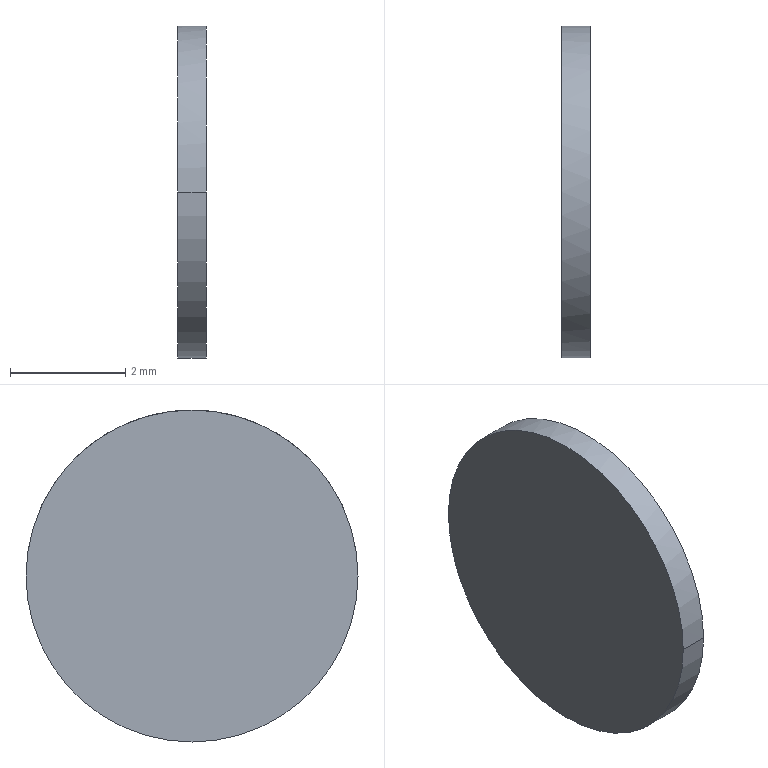Part | STEP file | _X2_7FC5724752A070ED7BA1_X0_1_8 | 1 solid | 4 faces | box 0.5 x 5.774 x 5.774 mm | volume 13.09 mm3 | cylinder 2 | plane 2 | commonest cylinder face diameters 5.774 x2
STEP:
#1=CARTESIAN_POINT('',(0.,0.,0.));
#2=DIRECTION('',(0.,0.,1.));
#3=DIRECTION('',(1.,0.,0.));
#4=AXIS2_PLACEMENT_3D('',#1,#2,#3);
#5=CARTESIAN_POINT('',(-43.5,-2.887,0.));
#6=VERTEX_POINT('',#5);
#7=CARTESIAN_POINT('',(-43.5,0.,2.887));
#8=VERTEX_POINT('',#7);
#9=CARTESIAN_POINT('',(-43.5,0.,0.));
#10=DIRECTION('',(-1.,0.,0.));
#11=DIRECTION('',(0.,-1.,0.));
#12=AXIS2_PLACEMENT_3D('',#9,#10,#11);
#13=CIRCLE('',#12,2.887);
#14=CARTESIAN_POINT('',(-43.5,0.,0.));
#15=DIRECTION('',(1.,0.,0.));
#16=DIRECTION('',(0.,1.,0.));
#17=AXIS2_PLACEMENT_3D('',#14,#15,#16);
#18=CYLINDRICAL_SURFACE('',#17,2.887);
#19=CARTESIAN_POINT('',(3.142,0.));
#20=DIRECTION('',(-1.,0.));
#21=VECTOR('',#20,1.);
#22=LINE('',#19,#21);
#23=(GEOMETRIC_REPRESENTATION_CONTEXT(2)PARAMETRIC_REPRESENTATION_CONTEXT()REPRESENTATION_CONTEXT('',''));
#24=DEFINITIONAL_REPRESENTATION('',(#22),#23);
#25=PCURVE('',#18,#24);
#26=CARTESIAN_POINT('',(-43.5,0.,0.));
#27=DIRECTION('',(-1.,0.,0.));
#28=DIRECTION('',(0.,-1.,0.));
#29=AXIS2_PLACEMENT_3D('',#26,#27,#28);
#30=PLANE('',#29);
#31=CARTESIAN_POINT('',(0.,0.));
#32=DIRECTION('',(1.,0.));
#33=AXIS2_PLACEMENT_2D('',#31,#32);
#34=CIRCLE('',#33,2.887);
#35=(GEOMETRIC_REPRESENTATION_CONTEXT(2)PARAMETRIC_REPRESENTATION_CONTEXT()REPRESENTATION_CONTEXT('',''));
#36=DEFINITIONAL_REPRESENTATION('',(#34),#35);
#37=PCURVE('',#30,#36);
#38=SURFACE_CURVE('',#13,(#25,#37),.PCURVE_S1.);
#39=EDGE_CURVE('',#6,#8,#38,.T.);
#40=ORIENTED_EDGE('',*,*,#39,.F.);
#41=CARTESIAN_POINT('',(-43.,-2.887,0.));
#42=VERTEX_POINT('',#41);
#43=CARTESIAN_POINT('',(-43.5,-2.887,0.));
#44=DIRECTION('',(1.,0.,0.));
#45=VECTOR('',#44,1.);
#46=LINE('',#43,#45);
#47=CARTESIAN_POINT('',(3.142,0.));
#48=DIRECTION('',(0.,1.));
#49=VECTOR('',#48,1.);
#50=LINE('',#47,#49);
#51=(GEOMETRIC_REPRESENTATION_CONTEXT(2)PARAMETRIC_REPRESENTATION_CONTEXT()REPRESENTATION_CONTEXT('',''));
#52=DEFINITIONAL_REPRESENTATION('',(#50),#51);
#53=PCURVE('',#18,#52);
#54=CARTESIAN_POINT('',(-43.5,0.,0.));
#55=DIRECTION('',(1.,0.,0.));
#56=DIRECTION('',(0.,1.,0.));
#57=AXIS2_PLACEMENT_3D('',#54,#55,#56);
#58=CYLINDRICAL_SURFACE('',#57,2.887);
#59=CARTESIAN_POINT('',(3.142,0.));
#60=DIRECTION('',(0.,1.));
#61=VECTOR('',#60,1.);
#62=LINE('',#59,#61);
#63=(GEOMETRIC_REPRESENTATION_CONTEXT(2)PARAMETRIC_REPRESENTATION_CONTEXT()REPRESENTATION_CONTEXT('',''));
#64=DEFINITIONAL_REPRESENTATION('',(#62),#63);
#65=PCURVE('',#58,#64);
#66=SURFACE_CURVE('',#46,(#53,#65),.PCURVE_S1.);
#67=EDGE_CURVE('',#6,#42,#66,.T.);
#68=ORIENTED_EDGE('',*,*,#67,.T.);
#69=CARTESIAN_POINT('',(-43.,2.887,0.));
#70=VERTEX_POINT('',#69);
#71=CARTESIAN_POINT('',(-43.,0.,0.));
#72=DIRECTION('',(1.,0.,0.));
#73=DIRECTION('',(0.,1.,0.));
#74=AXIS2_PLACEMENT_3D('',#71,#72,#73);
#75=CIRCLE('',#74,2.887);
#76=CARTESIAN_POINT('',(0.,0.5));
#77=DIRECTION('',(1.,0.));
#78=VECTOR('',#77,1.);
#79=LINE('',#76,#78);
#80=(GEOMETRIC_REPRESENTATION_CONTEXT(2)PARAMETRIC_REPRESENTATION_CONTEXT()REPRESENTATION_CONTEXT('',''));
#81=DEFINITIONAL_REPRESENTATION('',(#79),#80);
#82=PCURVE('',#18,#81);
#83=CARTESIAN_POINT('',(-43.,0.,0.));
#84=DIRECTION('',(-1.,0.,0.));
#85=DIRECTION('',(0.,-1.,0.));
#86=AXIS2_PLACEMENT_3D('',#83,#84,#85);
#87=PLANE('',#86);
#88=CARTESIAN_POINT('',(-2.887,0.));
#89=CARTESIAN_POINT('',(-2.887,5.));
#90=CARTESIAN_POINT('',(1.443,2.5));
#91=CARTESIAN_POINT('',(5.774,0.));
#92=CARTESIAN_POINT('',(1.443,-2.5));
#93=CARTESIAN_POINT('',(-2.887,-5.));
#94=CARTESIAN_POINT('',(-2.887,0.));
#95=(BOUNDED_CURVE()B_SPLINE_CURVE(2,(#88,#89,#90,#91,#92,#93,#94),.UNSPECIFIED.,.T.,.F.)B_SPLINE_CURVE_WITH_KNOTS((1,2,2,2,2,1),(-2.094,0.,2.094,4.189,6.283,8.378),.UNSPECIFIED.)CURVE()GEOMETRIC_REPRESENTATION_ITEM()RATIONAL_B_SPLINE_CURVE((1.,0.5,1.,0.5,1.,0.5,1.))REPRESENTATION_ITEM(''));
#96=(GEOMETRIC_REPRESENTATION_CONTEXT(2)PARAMETRIC_REPRESENTATION_CONTEXT()REPRESENTATION_CONTEXT('',''));
#97=DEFINITIONAL_REPRESENTATION('',(#95),#96);
#98=PCURVE('',#87,#97);
#99=SURFACE_CURVE('',#75,(#82,#98),.PCURVE_S1.);
#100=EDGE_CURVE('',#70,#42,#99,.T.);
#101=ORIENTED_EDGE('',*,*,#100,.F.);
#102=CARTESIAN_POINT('',(-43.5,2.887,0.));
#103=VERTEX_POINT('',#102);
#104=CARTESIAN_POINT('',(-43.5,2.887,0.));
#105=DIRECTION('',(1.,0.,0.));
#106=VECTOR('',#105,1.);
#107=LINE('',#104,#106);
#108=CARTESIAN_POINT('',(0.,0.));
#109=DIRECTION('',(0.,1.));
#110=VECTOR('',#109,1.);
#111=LINE('',#108,#110);
#112=(GEOMETRIC_REPRESENTATION_CONTEXT(2)PARAMETRIC_REPRESENTATION_CONTEXT()REPRESENTATION_CONTEXT('',''));
#113=DEFINITIONAL_REPRESENTATION('',(#111),#112);
#114=PCURVE('',#18,#113);
#115=CARTESIAN_POINT('',(6.283,0.));
#116=DIRECTION('',(0.,1.));
#117=VECTOR('',#116,1.);
#118=LINE('',#115,#117);
#119=(GEOMETRIC_REPRESENTATION_CONTEXT(2)PARAMETRIC_REPRESENTATION_CONTEXT()REPRESENTATION_CONTEXT('',''));
#120=DEFINITIONAL_REPRESENTATION('',(#118),#119);
#121=PCURVE('',#58,#120);
#122=SURFACE_CURVE('',#107,(#114,#121),.PCURVE_S1.);
#123=EDGE_CURVE('',#103,#70,#122,.T.);
#124=ORIENTED_EDGE('',*,*,#123,.F.);
#125=CARTESIAN_POINT('',(-43.5,0.,0.));
#126=DIRECTION('',(-1.,0.,0.));
#127=DIRECTION('',(0.,0.,1.));
#128=AXIS2_PLACEMENT_3D('',#125,#126,#127);
#129=CIRCLE('',#128,2.887);
#130=CARTESIAN_POINT('',(1.571,0.));
#131=DIRECTION('',(-1.,0.));
#132=VECTOR('',#131,1.);
#133=LINE('',#130,#132);
#134=(GEOMETRIC_REPRESENTATION_CONTEXT(2)PARAMETRIC_REPRESENTATION_CONTEXT()REPRESENTATION_CONTEXT('',''));
#135=DEFINITIONAL_REPRESENTATION('',(#133),#134);
#136=PCURVE('',#18,#135);
#137=CARTESIAN_POINT('',(0.,0.));
#138=DIRECTION('',(0.,1.));
#139=AXIS2_PLACEMENT_2D('',#137,#138);
#140=CIRCLE('',#139,2.887);
#141=(GEOMETRIC_REPRESENTATION_CONTEXT(2)PARAMETRIC_REPRESENTATION_CONTEXT()REPRESENTATION_CONTEXT('',''));
#142=DEFINITIONAL_REPRESENTATION('',(#140),#141);
#143=PCURVE('',#30,#142);
#144=SURFACE_CURVE('',#129,(#136,#143),.PCURVE_S1.);
#145=EDGE_CURVE('',#8,#103,#144,.T.);
#146=ORIENTED_EDGE('',*,*,#145,.F.);
#147=EDGE_LOOP('',(#40,#68,#101,#124,#146));
#148=FACE_BOUND('',#147,.T.);
#149=ADVANCED_FACE('',(#148),#18,.T.);
#150=CARTESIAN_POINT('',(-43.5,0.,-2.887));
#151=VERTEX_POINT('',#150);
#152=CARTESIAN_POINT('',(-43.5,0.,0.));
#153=DIRECTION('',(-1.,0.,0.));
#154=DIRECTION('',(0.,0.,-1.));
#155=AXIS2_PLACEMENT_3D('',#152,#153,#154);
#156=CIRCLE('',#155,2.887);
#157=CARTESIAN_POINT('',(0.,0.));
#158=DIRECTION('',(0.,-1.));
#159=AXIS2_PLACEMENT_2D('',#157,#158);
#160=CIRCLE('',#159,2.887);
#161=(GEOMETRIC_REPRESENTATION_CONTEXT(2)PARAMETRIC_REPRESENTATION_CONTEXT()REPRESENTATION_CONTEXT('',''));
#162=DEFINITIONAL_REPRESENTATION('',(#160),#161);
#163=PCURVE('',#30,#162);
#164=CARTESIAN_POINT('',(4.712,0.));
#165=DIRECTION('',(-1.,0.));
#166=VECTOR('',#165,1.);
#167=LINE('',#164,#166);
#168=(GEOMETRIC_REPRESENTATION_CONTEXT(2)PARAMETRIC_REPRESENTATION_CONTEXT()REPRESENTATION_CONTEXT('',''));
#169=DEFINITIONAL_REPRESENTATION('',(#167),#168);
#170=PCURVE('',#58,#169);
#171=SURFACE_CURVE('',#156,(#163,#170),.PCURVE_S1.);
#172=EDGE_CURVE('',#151,#6,#171,.T.);
#173=ORIENTED_EDGE('',*,*,#172,.F.);
#174=CARTESIAN_POINT('',(-43.5,0.,0.));
#175=DIRECTION('',(-1.,0.,0.));
#176=DIRECTION('',(0.,1.,0.));
#177=AXIS2_PLACEMENT_3D('',#174,#175,#176);
#178=CIRCLE('',#177,2.887);
#179=CARTESIAN_POINT('',(0.,0.));
#180=DIRECTION('',(-1.,0.));
#181=AXIS2_PLACEMENT_2D('',#179,#180);
#182=CIRCLE('',#181,2.887);
#183=(GEOMETRIC_REPRESENTATION_CONTEXT(2)PARAMETRIC_REPRESENTATION_CONTEXT()REPRESENTATION_CONTEXT('',''));
#184=DEFINITIONAL_REPRESENTATION('',(#182),#183);
#185=PCURVE('',#30,#184);
#186=CARTESIAN_POINT('',(6.283,0.));
#187=DIRECTION('',(-1.,0.));
#188=VECTOR('',#187,1.);
#189=LINE('',#186,#188);
#190=(GEOMETRIC_REPRESENTATION_CONTEXT(2)PARAMETRIC_REPRESENTATION_CONTEXT()REPRESENTATION_CONTEXT('',''));
#191=DEFINITIONAL_REPRESENTATION('',(#189),#190);
#192=PCURVE('',#58,#191);
#193=SURFACE_CURVE('',#178,(#185,#192),.PCURVE_S1.);
#194=EDGE_CURVE('',#103,#151,#193,.T.);
#195=ORIENTED_EDGE('',*,*,#194,.F.);
#196=ORIENTED_EDGE('',*,*,#145,.F.);
#197=ORIENTED_EDGE('',*,*,#39,.F.);
#198=EDGE_LOOP('',(#173,#195,#196,#197));
#199=FACE_BOUND('',#198,.F.);
#200=ADVANCED_FACE('',(#199),#30,.T.);
#201=ORIENTED_EDGE('',*,*,#123,.T.);
#202=CARTESIAN_POINT('',(-43.,0.,-2.887));
#203=VERTEX_POINT('',#202);
#204=CARTESIAN_POINT('',(-43.,0.,0.));
#205=DIRECTION('',(1.,0.,0.));
#206=DIRECTION('',(0.,0.,-1.));
#207=AXIS2_PLACEMENT_3D('',#204,#205,#206);
#208=CIRCLE('',#207,2.887);
#209=CARTESIAN_POINT('',(4.712,0.5));
#210=DIRECTION('',(1.,0.));
#211=VECTOR('',#210,1.);
#212=LINE('',#209,#211);
#213=(GEOMETRIC_REPRESENTATION_CONTEXT(2)PARAMETRIC_REPRESENTATION_CONTEXT()REPRESENTATION_CONTEXT('',''));
#214=DEFINITIONAL_REPRESENTATION('',(#212),#213);
#215=PCURVE('',#58,#214);
#216=CARTESIAN_POINT('',(0.,-2.887));
#217=CARTESIAN_POINT('',(-5.,-2.887));
#218=CARTESIAN_POINT('',(-2.5,1.443));
#219=CARTESIAN_POINT('',(0.,5.774));
#220=CARTESIAN_POINT('',(2.5,1.443));
#221=CARTESIAN_POINT('',(5.,-2.887));
#222=CARTESIAN_POINT('',(0.,-2.887));
#223=(BOUNDED_CURVE()B_SPLINE_CURVE(2,(#216,#217,#218,#219,#220,#221,#222),.UNSPECIFIED.,.T.,.F.)B_SPLINE_CURVE_WITH_KNOTS((1,2,2,2,2,1),(-2.094,0.,2.094,4.189,6.283,8.378),.UNSPECIFIED.)CURVE()GEOMETRIC_REPRESENTATION_ITEM()RATIONAL_B_SPLINE_CURVE((1.,0.5,1.,0.5,1.,0.5,1.))REPRESENTATION_ITEM(''));
#224=(GEOMETRIC_REPRESENTATION_CONTEXT(2)PARAMETRIC_REPRESENTATION_CONTEXT()REPRESENTATION_CONTEXT('',''));
#225=DEFINITIONAL_REPRESENTATION('',(#223),#224);
#226=PCURVE('',#87,#225);
#227=SURFACE_CURVE('',#208,(#215,#226),.PCURVE_S1.);
#228=EDGE_CURVE('',#203,#70,#227,.T.);
#229=ORIENTED_EDGE('',*,*,#228,.F.);
#230=CARTESIAN_POINT('',(-43.,0.,0.));
#231=DIRECTION('',(1.,0.,0.));
#232=DIRECTION('',(0.,-1.,0.));
#233=AXIS2_PLACEMENT_3D('',#230,#231,#232);
#234=CIRCLE('',#233,2.887);
#235=CARTESIAN_POINT('',(3.142,0.5));
#236=DIRECTION('',(1.,0.));
#237=VECTOR('',#236,1.);
#238=LINE('',#235,#237);
#239=(GEOMETRIC_REPRESENTATION_CONTEXT(2)PARAMETRIC_REPRESENTATION_CONTEXT()REPRESENTATION_CONTEXT('',''));
#240=DEFINITIONAL_REPRESENTATION('',(#238),#239);
#241=PCURVE('',#58,#240);
#242=CARTESIAN_POINT('',(2.887,0.));
#243=CARTESIAN_POINT('',(2.887,-5.));
#244=CARTESIAN_POINT('',(-1.443,-2.5));
#245=CARTESIAN_POINT('',(-5.774,0.));
#246=CARTESIAN_POINT('',(-1.443,2.5));
#247=CARTESIAN_POINT('',(2.887,5.));
#248=CARTESIAN_POINT('',(2.887,0.));
#249=(BOUNDED_CURVE()B_SPLINE_CURVE(2,(#242,#243,#244,#245,#246,#247,#248),.UNSPECIFIED.,.T.,.F.)B_SPLINE_CURVE_WITH_KNOTS((1,2,2,2,2,1),(-2.094,0.,2.094,4.189,6.283,8.378),.UNSPECIFIED.)CURVE()GEOMETRIC_REPRESENTATION_ITEM()RATIONAL_B_SPLINE_CURVE((1.,0.5,1.,0.5,1.,0.5,1.))REPRESENTATION_ITEM(''));
#250=(GEOMETRIC_REPRESENTATION_CONTEXT(2)PARAMETRIC_REPRESENTATION_CONTEXT()REPRESENTATION_CONTEXT('',''));
#251=DEFINITIONAL_REPRESENTATION('',(#249),#250);
#252=PCURVE('',#87,#251);
#253=SURFACE_CURVE('',#234,(#241,#252),.PCURVE_S1.);
#254=EDGE_CURVE('',#42,#203,#253,.T.);
#255=ORIENTED_EDGE('',*,*,#254,.F.);
#256=ORIENTED_EDGE('',*,*,#67,.F.);
#257=ORIENTED_EDGE('',*,*,#172,.F.);
#258=ORIENTED_EDGE('',*,*,#194,.F.);
#259=EDGE_LOOP('',(#201,#229,#255,#256,#257,#258));
#260=FACE_BOUND('',#259,.T.);
#261=ADVANCED_FACE('',(#260),#58,.T.);
#262=ORIENTED_EDGE('',*,*,#228,.F.);
#263=ORIENTED_EDGE('',*,*,#254,.F.);
#264=ORIENTED_EDGE('',*,*,#100,.F.);
#265=EDGE_LOOP('',(#262,#263,#264));
#266=FACE_BOUND('',#265,.F.);
#267=ADVANCED_FACE('',(#266),#87,.F.);
#268=CLOSED_SHELL('',(#149,#200,#261,#267));
#269=MANIFOLD_SOLID_BREP('',#268);
#270=(LENGTH_UNIT()NAMED_UNIT(*)SI_UNIT(.MILLI.,.METRE.));
#271=UNCERTAINTY_MEASURE_WITH_UNIT(LENGTH_MEASURE(0.0000001),#270,'','');
#272=(NAMED_UNIT(*)PLANE_ANGLE_UNIT()SI_UNIT($,.RADIAN.));
#273=(NAMED_UNIT(*)SI_UNIT($,.STERADIAN.)SOLID_ANGLE_UNIT());
#274=(GEOMETRIC_REPRESENTATION_CONTEXT(3)GLOBAL_UNCERTAINTY_ASSIGNED_CONTEXT((#271))GLOBAL_UNIT_ASSIGNED_CONTEXT((#270,#272,#273))REPRESENTATION_CONTEXT('',''));
#275=ADVANCED_BREP_SHAPE_REPRESENTATION('',(#4,#269),#274);